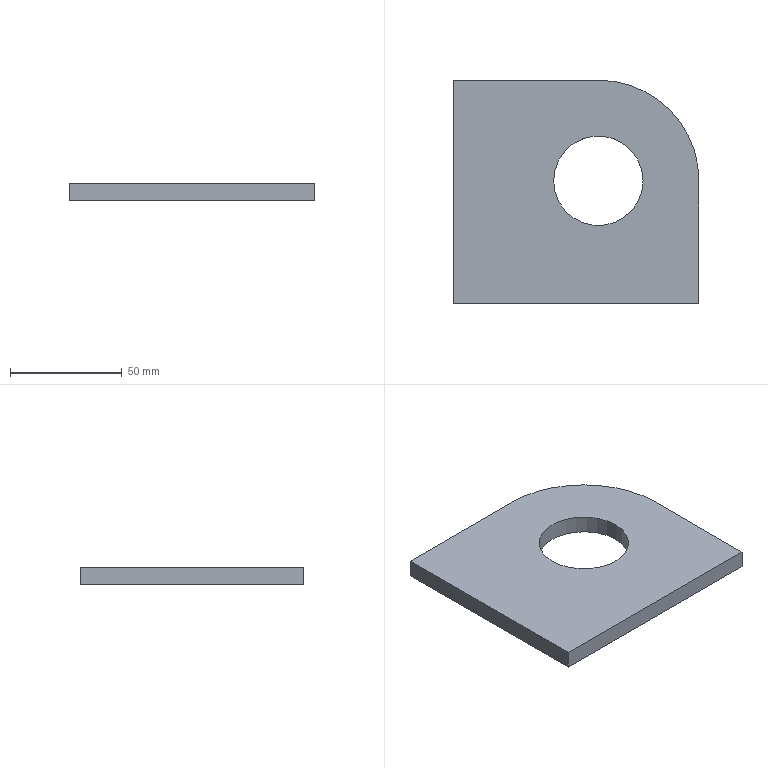Part | SolidWorks | features Extrusion 1 | 1 solid | 9 faces | box 110 x 100 x 8 mm | volume 74470 mm3 | plane 6 | cylinder 3 | commonest cylinder face diameters 40 x2 90 x1
STEP:
#1=CARTESIAN_POINT('',(45.,55.,8.));
#2=VERTEX_POINT('',#1);
#3=CARTESIAN_POINT('',(85.,55.,8.));
#4=VERTEX_POINT('',#3);
#5=CARTESIAN_POINT('',(65.,55.,8.));
#6=DIRECTION('',(0.,0.,1.));
#7=DIRECTION('',(1.,0.,0.));
#8=AXIS2_PLACEMENT_3D('',#5,#6,#7);
#9=CIRCLE('',#8,20.);
#10=EDGE_CURVE('',#2,#4,#9,.T.);
#11=ORIENTED_EDGE('',*,*,#10,.T.);
#12=CARTESIAN_POINT('',(85.,55.,0.));
#13=VERTEX_POINT('',#12);
#14=CARTESIAN_POINT('',(85.,55.,8.));
#15=DIRECTION('',(0.,0.,-1.));
#16=VECTOR('',#15,1000.);
#17=LINE('',#14,#16);
#18=EDGE_CURVE('',#4,#13,#17,.T.);
#19=ORIENTED_EDGE('',*,*,#18,.T.);
#20=CARTESIAN_POINT('',(45.,55.,0.));
#21=VERTEX_POINT('',#20);
#22=CARTESIAN_POINT('',(65.,55.,0.));
#23=DIRECTION('',(0.,0.,1.));
#24=DIRECTION('',(1.,0.,0.));
#25=AXIS2_PLACEMENT_3D('',#22,#23,#24);
#26=CIRCLE('',#25,20.);
#27=EDGE_CURVE('',#21,#13,#26,.T.);
#28=ORIENTED_EDGE('',*,*,#27,.F.);
#29=CARTESIAN_POINT('',(45.,55.,8.));
#30=DIRECTION('',(0.,0.,-1.));
#31=VECTOR('',#30,1000.);
#32=LINE('',#29,#31);
#33=EDGE_CURVE('',#2,#21,#32,.T.);
#34=ORIENTED_EDGE('',*,*,#33,.F.);
#35=EDGE_LOOP('',(#11,#19,#28,#34));
#36=FACE_OUTER_BOUND('',#35,.T.);
#37=CARTESIAN_POINT('',(65.,55.,8.));
#38=DIRECTION('',(0.,0.,-1.));
#39=DIRECTION('',(-1.,0.,0.));
#40=AXIS2_PLACEMENT_3D('',#37,#38,#39);
#41=CYLINDRICAL_SURFACE('',#40,20.);
#42=ADVANCED_FACE('',(#36),#41,.F.);
#43=CARTESIAN_POINT('',(0.,100.,8.));
#44=VERTEX_POINT('',#43);
#45=CARTESIAN_POINT('',(0.,0.,8.));
#46=VERTEX_POINT('',#45);
#47=CARTESIAN_POINT('',(0.,0.,8.));
#48=DIRECTION('',(0.,-1.,0.));
#49=VECTOR('',#48,1000.);
#50=LINE('',#47,#49);
#51=EDGE_CURVE('',#44,#46,#50,.T.);
#52=ORIENTED_EDGE('',*,*,#51,.T.);
#53=CARTESIAN_POINT('',(110.,0.,8.));
#54=VERTEX_POINT('',#53);
#55=CARTESIAN_POINT('',(0.,0.,8.));
#56=DIRECTION('',(1.,0.,0.));
#57=VECTOR('',#56,1000.);
#58=LINE('',#55,#57);
#59=EDGE_CURVE('',#46,#54,#58,.T.);
#60=ORIENTED_EDGE('',*,*,#59,.T.);
#61=CARTESIAN_POINT('',(110.,55.,8.));
#62=VERTEX_POINT('',#61);
#63=CARTESIAN_POINT('',(110.,0.,8.));
#64=DIRECTION('',(0.,1.,0.));
#65=VECTOR('',#64,1000.);
#66=LINE('',#63,#65);
#67=EDGE_CURVE('',#54,#62,#66,.T.);
#68=ORIENTED_EDGE('',*,*,#67,.T.);
#69=CARTESIAN_POINT('',(65.,100.,8.));
#70=VERTEX_POINT('',#69);
#71=CARTESIAN_POINT('',(65.,55.,8.));
#72=DIRECTION('',(0.,0.,1.));
#73=DIRECTION('',(-1.,0.,0.));
#74=AXIS2_PLACEMENT_3D('',#71,#72,#73);
#75=CIRCLE('',#74,45.);
#76=EDGE_CURVE('',#62,#70,#75,.T.);
#77=ORIENTED_EDGE('',*,*,#76,.T.);
#78=CARTESIAN_POINT('',(0.,100.,8.));
#79=DIRECTION('',(-1.,0.,0.));
#80=VECTOR('',#79,1000.);
#81=LINE('',#78,#80);
#82=EDGE_CURVE('',#70,#44,#81,.T.);
#83=ORIENTED_EDGE('',*,*,#82,.T.);
#84=EDGE_LOOP('',(#52,#60,#68,#77,#83));
#85=FACE_OUTER_BOUND('',#84,.T.);
#86=ORIENTED_EDGE('',*,*,#10,.F.);
#87=CARTESIAN_POINT('',(65.,55.,8.));
#88=DIRECTION('',(0.,0.,1.));
#89=DIRECTION('',(1.,0.,0.));
#90=AXIS2_PLACEMENT_3D('',#87,#88,#89);
#91=CIRCLE('',#90,20.);
#92=EDGE_CURVE('',#4,#2,#91,.T.);
#93=ORIENTED_EDGE('',*,*,#92,.F.);
#94=EDGE_LOOP('',(#86,#93));
#95=FACE_BOUND('',#94,.T.);
#96=CARTESIAN_POINT('',(65.,55.,8.));
#97=DIRECTION('',(0.,0.,-1.));
#98=DIRECTION('',(-1.,0.,0.));
#99=AXIS2_PLACEMENT_3D('',#96,#97,#98);
#100=PLANE('',#99);
#101=ADVANCED_FACE('',(#85,#95),#100,.F.);
#102=CARTESIAN_POINT('',(0.,100.,0.));
#103=VERTEX_POINT('',#102);
#104=CARTESIAN_POINT('',(0.,0.,0.));
#105=VERTEX_POINT('',#104);
#106=CARTESIAN_POINT('',(0.,0.,0.));
#107=DIRECTION('',(0.,-1.,0.));
#108=VECTOR('',#107,1000.);
#109=LINE('',#106,#108);
#110=EDGE_CURVE('',#103,#105,#109,.T.);
#111=ORIENTED_EDGE('',*,*,#110,.F.);
#112=CARTESIAN_POINT('',(65.,100.,0.));
#113=VERTEX_POINT('',#112);
#114=CARTESIAN_POINT('',(0.,100.,0.));
#115=DIRECTION('',(-1.,0.,0.));
#116=VECTOR('',#115,1000.);
#117=LINE('',#114,#116);
#118=EDGE_CURVE('',#113,#103,#117,.T.);
#119=ORIENTED_EDGE('',*,*,#118,.F.);
#120=CARTESIAN_POINT('',(110.,55.,0.));
#121=VERTEX_POINT('',#120);
#122=CARTESIAN_POINT('',(65.,55.,0.));
#123=DIRECTION('',(0.,0.,1.));
#124=DIRECTION('',(-1.,0.,0.));
#125=AXIS2_PLACEMENT_3D('',#122,#123,#124);
#126=CIRCLE('',#125,45.);
#127=EDGE_CURVE('',#121,#113,#126,.T.);
#128=ORIENTED_EDGE('',*,*,#127,.F.);
#129=CARTESIAN_POINT('',(110.,0.,0.));
#130=VERTEX_POINT('',#129);
#131=CARTESIAN_POINT('',(110.,0.,0.));
#132=DIRECTION('',(0.,1.,0.));
#133=VECTOR('',#132,1000.);
#134=LINE('',#131,#133);
#135=EDGE_CURVE('',#130,#121,#134,.T.);
#136=ORIENTED_EDGE('',*,*,#135,.F.);
#137=CARTESIAN_POINT('',(0.,0.,0.));
#138=DIRECTION('',(1.,0.,0.));
#139=VECTOR('',#138,1000.);
#140=LINE('',#137,#139);
#141=EDGE_CURVE('',#105,#130,#140,.T.);
#142=ORIENTED_EDGE('',*,*,#141,.F.);
#143=EDGE_LOOP('',(#111,#119,#128,#136,#142));
#144=FACE_OUTER_BOUND('',#143,.T.);
#145=ORIENTED_EDGE('',*,*,#27,.T.);
#146=CARTESIAN_POINT('',(65.,55.,0.));
#147=DIRECTION('',(0.,0.,1.));
#148=DIRECTION('',(1.,0.,0.));
#149=AXIS2_PLACEMENT_3D('',#146,#147,#148);
#150=CIRCLE('',#149,20.);
#151=EDGE_CURVE('',#13,#21,#150,.T.);
#152=ORIENTED_EDGE('',*,*,#151,.T.);
#153=EDGE_LOOP('',(#145,#152));
#154=FACE_BOUND('',#153,.T.);
#155=CARTESIAN_POINT('',(65.,55.,0.));
#156=DIRECTION('',(0.,0.,-1.));
#157=DIRECTION('',(-1.,0.,0.));
#158=AXIS2_PLACEMENT_3D('',#155,#156,#157);
#159=PLANE('',#158);
#160=ADVANCED_FACE('',(#144,#154),#159,.T.);
#161=ORIENTED_EDGE('',*,*,#110,.T.);
#162=CARTESIAN_POINT('',(0.,0.,8.));
#163=DIRECTION('',(0.,0.,-1.));
#164=VECTOR('',#163,1000.);
#165=LINE('',#162,#164);
#166=EDGE_CURVE('',#46,#105,#165,.T.);
#167=ORIENTED_EDGE('',*,*,#166,.F.);
#168=ORIENTED_EDGE('',*,*,#51,.F.);
#169=CARTESIAN_POINT('',(0.,100.,8.));
#170=DIRECTION('',(0.,0.,-1.));
#171=VECTOR('',#170,1000.);
#172=LINE('',#169,#171);
#173=EDGE_CURVE('',#44,#103,#172,.T.);
#174=ORIENTED_EDGE('',*,*,#173,.T.);
#175=EDGE_LOOP('',(#161,#167,#168,#174));
#176=FACE_OUTER_BOUND('',#175,.T.);
#177=CARTESIAN_POINT('',(0.,0.,8.));
#178=DIRECTION('',(1.,0.,0.));
#179=DIRECTION('',(0.,0.,-1.));
#180=AXIS2_PLACEMENT_3D('',#177,#178,#179);
#181=PLANE('',#180);
#182=ADVANCED_FACE('',(#176),#181,.F.);
#183=ORIENTED_EDGE('',*,*,#141,.T.);
#184=CARTESIAN_POINT('',(110.,0.,8.));
#185=DIRECTION('',(0.,0.,-1.));
#186=VECTOR('',#185,1000.);
#187=LINE('',#184,#186);
#188=EDGE_CURVE('',#54,#130,#187,.T.);
#189=ORIENTED_EDGE('',*,*,#188,.F.);
#190=ORIENTED_EDGE('',*,*,#59,.F.);
#191=ORIENTED_EDGE('',*,*,#166,.T.);
#192=EDGE_LOOP('',(#183,#189,#190,#191));
#193=FACE_OUTER_BOUND('',#192,.T.);
#194=CARTESIAN_POINT('',(0.,0.,8.));
#195=DIRECTION('',(0.,1.,0.));
#196=DIRECTION('',(0.,0.,1.));
#197=AXIS2_PLACEMENT_3D('',#194,#195,#196);
#198=PLANE('',#197);
#199=ADVANCED_FACE('',(#193),#198,.F.);
#200=ORIENTED_EDGE('',*,*,#135,.T.);
#201=CARTESIAN_POINT('',(110.,55.,8.));
#202=DIRECTION('',(0.,0.,-1.));
#203=VECTOR('',#202,1000.);
#204=LINE('',#201,#203);
#205=EDGE_CURVE('',#62,#121,#204,.T.);
#206=ORIENTED_EDGE('',*,*,#205,.F.);
#207=ORIENTED_EDGE('',*,*,#67,.F.);
#208=ORIENTED_EDGE('',*,*,#188,.T.);
#209=EDGE_LOOP('',(#200,#206,#207,#208));
#210=FACE_OUTER_BOUND('',#209,.T.);
#211=CARTESIAN_POINT('',(110.,0.,8.));
#212=DIRECTION('',(-1.,0.,0.));
#213=DIRECTION('',(0.,0.,1.));
#214=AXIS2_PLACEMENT_3D('',#211,#212,#213);
#215=PLANE('',#214);
#216=ADVANCED_FACE('',(#210),#215,.F.);
#217=ORIENTED_EDGE('',*,*,#127,.T.);
#218=CARTESIAN_POINT('',(65.,100.,8.));
#219=DIRECTION('',(0.,0.,-1.));
#220=VECTOR('',#219,1000.);
#221=LINE('',#218,#220);
#222=EDGE_CURVE('',#70,#113,#221,.T.);
#223=ORIENTED_EDGE('',*,*,#222,.F.);
#224=ORIENTED_EDGE('',*,*,#76,.F.);
#225=ORIENTED_EDGE('',*,*,#205,.T.);
#226=EDGE_LOOP('',(#217,#223,#224,#225));
#227=FACE_OUTER_BOUND('',#226,.T.);
#228=CARTESIAN_POINT('',(65.,55.,8.));
#229=DIRECTION('',(0.,0.,-1.));
#230=DIRECTION('',(-1.,0.,0.));
#231=AXIS2_PLACEMENT_3D('',#228,#229,#230);
#232=CYLINDRICAL_SURFACE('',#231,45.);
#233=ADVANCED_FACE('',(#227),#232,.T.);
#234=ORIENTED_EDGE('',*,*,#118,.T.);
#235=ORIENTED_EDGE('',*,*,#173,.F.);
#236=ORIENTED_EDGE('',*,*,#82,.F.);
#237=ORIENTED_EDGE('',*,*,#222,.T.);
#238=EDGE_LOOP('',(#234,#235,#236,#237));
#239=FACE_OUTER_BOUND('',#238,.T.);
#240=CARTESIAN_POINT('',(0.,100.,8.));
#241=DIRECTION('',(0.,-1.,0.));
#242=DIRECTION('',(0.,0.,-1.));
#243=AXIS2_PLACEMENT_3D('',#240,#241,#242);
#244=PLANE('',#243);
#245=ADVANCED_FACE('',(#239),#244,.F.);
#246=ORIENTED_EDGE('',*,*,#18,.F.);
#247=ORIENTED_EDGE('',*,*,#92,.T.);
#248=ORIENTED_EDGE('',*,*,#33,.T.);
#249=ORIENTED_EDGE('',*,*,#151,.F.);
#250=EDGE_LOOP('',(#246,#247,#248,#249));
#251=FACE_OUTER_BOUND('',#250,.T.);
#252=CARTESIAN_POINT('',(65.,55.,8.));
#253=DIRECTION('',(0.,0.,-1.));
#254=DIRECTION('',(-1.,0.,0.));
#255=AXIS2_PLACEMENT_3D('',#252,#253,#254);
#256=CYLINDRICAL_SURFACE('',#255,20.);
#257=ADVANCED_FACE('',(#251),#256,.F.);
#258=CLOSED_SHELL('',(#42,#101,#160,#182,#199,#216,#233,#245,#257));
#259=MANIFOLD_SOLID_BREP('',#258);
#260=CARTESIAN_POINT('',(0.,0.,0.));
#261=DIRECTION('',(0.,0.,1.));
#262=DIRECTION('',(1.,0.,0.));
#263=AXIS2_PLACEMENT_3D('',#260,#261,#262);
#264=(LENGTH_UNIT()NAMED_UNIT(*)SI_UNIT(.MILLI.,.METRE.));
#265=UNCERTAINTY_MEASURE_WITH_UNIT(LENGTH_MEASURE(0.00001),#264,'','');
#266=(NAMED_UNIT(*)PLANE_ANGLE_UNIT()SI_UNIT($,.RADIAN.));
#267=(NAMED_UNIT(*)SI_UNIT($,.STERADIAN.)SOLID_ANGLE_UNIT());
#268=(GEOMETRIC_REPRESENTATION_CONTEXT(3)GLOBAL_UNCERTAINTY_ASSIGNED_CONTEXT((#265))GLOBAL_UNIT_ASSIGNED_CONTEXT((#264,#266,#267))REPRESENTATION_CONTEXT('',''));
#269=ADVANCED_BREP_SHAPE_REPRESENTATION('',(#259,#263),#268);